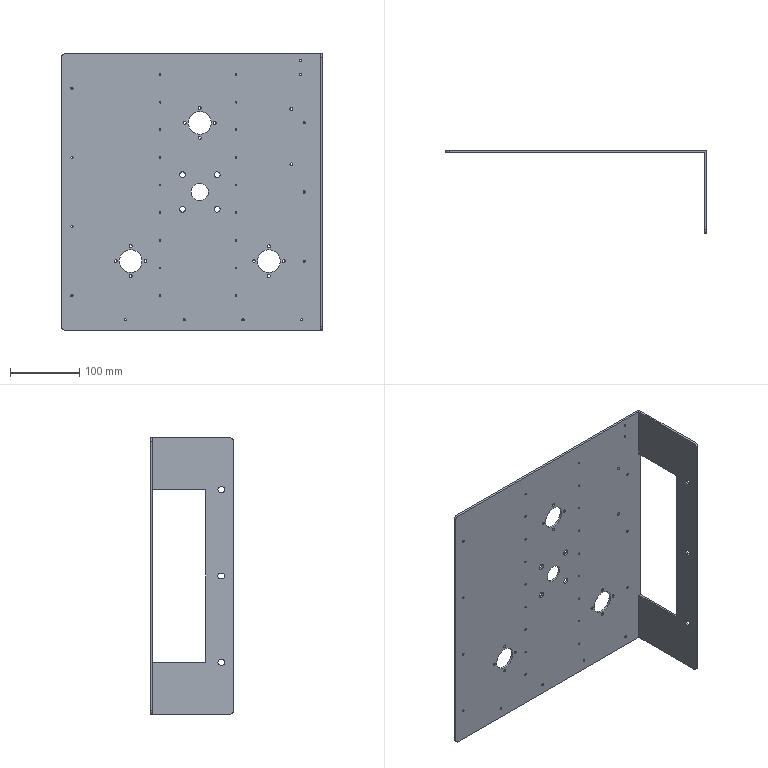Part | SolidWorks | features HoleWzd 10, ICE 3, FlattenBends 2, MoveFace 2, ProcessBends 2, BossThin 1, Extrusion 1, Fillet 1, LPattern 1 | 1 solid | 133 faces | box 377.5 x 120 x 400 mm | volume 523953 mm3 | cylinder 116 | plane 17 | commonest cylinder face diameters 2.5 x36 3.2 x26 4.2 x24 8.6 x8 8.2 x6 33 x6